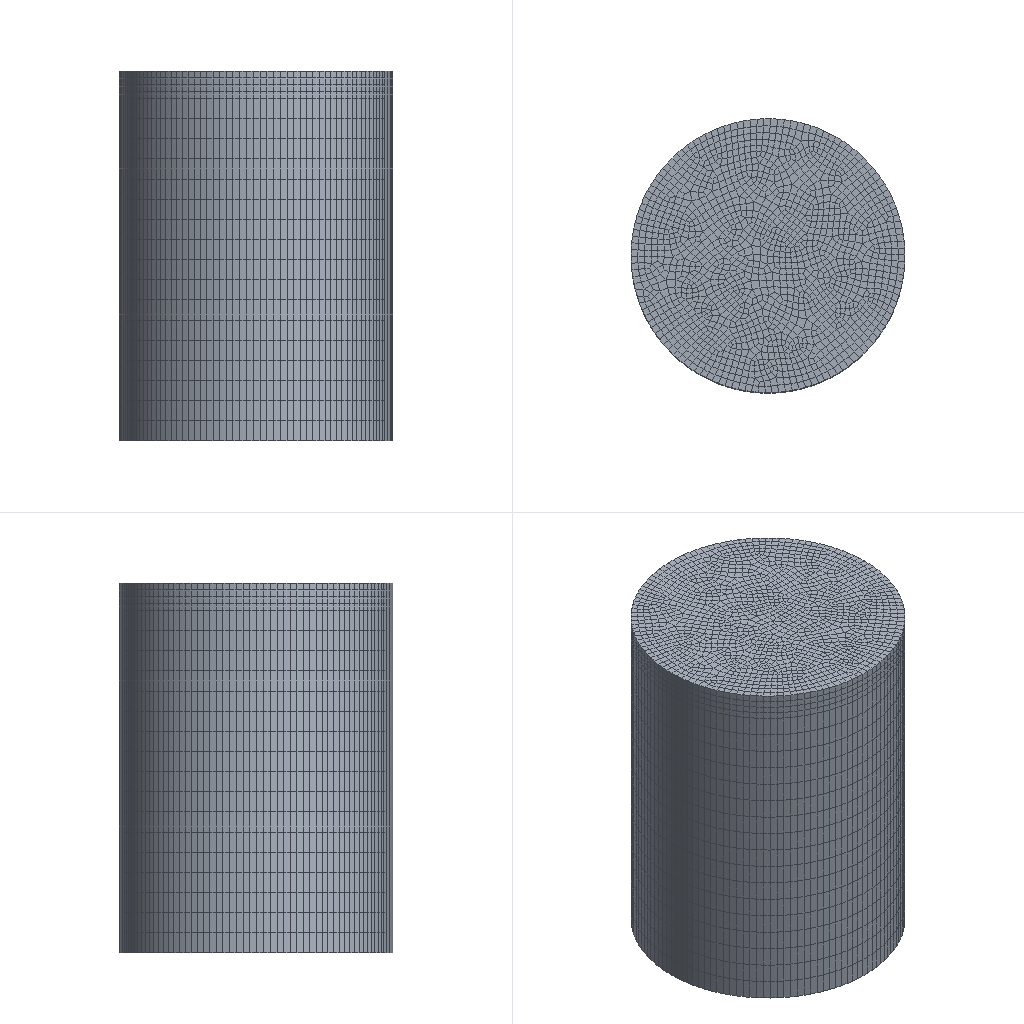Simulation study | abaqus
Set-up summary:
category,name,step,type,value,unit,region
solver,abaqus
solver,version,,,Abaqus/Explicit 2020
units,not stated in the deck,,not stated
analysis,deck,,transient,transient
load_step,Step-1,Step-1,transient
load_step,requested,,,1
mesh,nodes,,,37413
mesh,elements,,,34494
element_type,R3D3,,rigid,192
element_type,R3D4,,rigid,618
element_type,C3D8R,,solid,33684
load,load commands in deck,,count,2
bc,support commands in deck,,count,7
material,AL,,in results
material,CFRP-COPY,,in results
check,setup vs results,,match,"per instance, exact: element labels, types and connectivity; labels of the nodes the elements use; coordinates not compared"
Abaqus input file, long lists of numbers shortened:
*Heading
** Job name: Job-2 Model name: Model-1-Copy
** Generated by: Abaqus/CAE 2020
*Preprint, echo=NO, model=NO, history=NO, contact=NO
**
** PARTS
**
*Part, name=work
*Node
      1,   1.6,  -1.2,   5.2
      2,   1.6,  -1.2,    5.1
** (36694 more lines like these left out)
*Element, type=C3D8R
   1, 1117, 1163, 1135, 1050, 2659, 2705, 2677, 2592
   2,   81, 1117, 1050,   80,  206, 2659, 2592,  205
** (33682 more lines like these left out)
*Nset, nset=Set-18
     3,     4,   257,   258,   259,   260,   261,   262,   263,   264,   265,   266,   267,   268,   269,   270
   271,   272,   273,   274,   275,   276,   277,   278,   279,   280,   281,   282,   283,   284,   285,   286
** (1875 more lines like these left out)
*Elset, elset=Set-18, generate
  3209,  30476,      1
*Nset, nset=Set-17
     1,     2,     5,     6,     7,     8,     9,    10,    11,    12,    13,    14,    15,    16,    17,    18
    19,    20,    21,    22,    23,    24,    25,    26,    27,    28,    29,    30,    31,    32,    33,    34
** (415 more lines like these left out)
*Elset, elset=Set-17
     1,     2,     3,     4,     5,     6,     7,     8,     9,    10,    11,    12,    13,    14,    15,    16
    17,    18,    19,    20,    21,    22,    23,    24,    25,    26,    27,    28,    29,    30,    31,    32
** (299 more lines like these left out)
*Nset, nset=Set-19
     1,     2,     3,     5,     6,     7,     8,     9,    10,    11,    12,    13,    14,    15,    16,    17
    18,    19,    20,    21,    22,    23,    24,    25,    26,    27,    28,    29,    30,    31,    32,    33
** (520 more lines like these left out)
*Elset, elset=Set-19
     1,     2,     3,     4,     5,     6,     7,     8,     9,    10,    11,    12,    13,    14,    15,    16
    17,    18,    19,    20,    21,    22,    23,    24,    25,    26,    27,    28,    29,    30,    31,    32
** (399 more lines like these left out)
** Section: Section-2
*Solid Section, elset=Set-19, material=cfrp-Copy
,
** Section: al
*Solid Section, elset=Set-18, material=al
,
*End Part
**
*Part, name=zuantou_tool
*Node
      1,   0.8975, -0.3369,  0.4764
      2,  0.9447, -0.3279,  0.4373
** (714 more lines like these left out)
*Element, type=R3D4
 1,  1,  2, 34, 73
 2, 73, 34, 35, 72
** (616 more lines like these left out)
*Element, type=R3D3
371,  15,   4, 522
372, 537, 524, 527
** (190 more lines like these left out)
*Node
    717, -1.66533454e-16, -5.55111512e-17,   10.601
*Nset, nset=zuantou_tool-RefPt_, internal
717,
*Elset, elset=zuantou_tool, generate
   1,  810,    1
*End Part
**
**
** ASSEMBLY
**
*Assembly, name=Assembly
**
*Instance, name=work-1, part=work
*End Instance
**
*Instance, name=zuantou_tool-1, part=zuantou_tool
          0.,           0.,          5.4
*End Instance
**
*Node
      1,           0., 1.22464685e-16,           0.
*Nset, nset=Set-2, instance=zuantou_tool-1
 717,
*Nset, nset=Set-3, instance=zuantou_tool-1
 717,
*Nset, nset=Set-5, instance=zuantou_tool-1
 717,
*Nset, nset=Set-6, instance=work-1
    4,  382,  383,  384,  385,  386,  387,  388,  389,  390,  391,  392,  393,  394,  395,  396
  397,  398,  399,  400,  401,  402,  403,  404,  405,  406,  407,  408,  409,  410,  411,  412
** (103 more lines like these left out)
*Elset, elset=Set-6, instance=work-1, generate
 28873,  30476,      1
*Nset, nset=Set-7, instance=zuantou_tool-1
 717,
*Nset, nset=Set-11, instance=work-1
    4,  382,  383,  384,  385,  386,  387,  388,  389,  390,  391,  392,  393,  394,  395,  396
  397,  398,  399,  400,  401,  402,  403,  404,  405,  406,  407,  408,  409,  410,  411,  412
** (103 more lines like these left out)
*Elset, elset=Set-11, instance=work-1, generate
 28873,  30476,      1
*Nset, nset=m_Set-9
 1,
*Nset, nset=rp-fix
 1,
*Nset, nset=s_Set-4, instance=work-1
   4,   6, 382, 383, 384, 385, 386, 387, 388, 389, 390, 391, 392, 393, 394, 395
 396, 397, 398, 399, 400, 401, 402, 403, 404, 405, 406, 407, 408, 409, 410, 411
** (6 more lines like these left out)
*Elset, elset=s_Set-4, instance=work-1
 28874, 28885, 28888, 28900, 28901, 28912, 28913, 28922, 28923, 28926, 28927, 28928, 28934, 28947, 28950, 28951
 28952, 28954, 28966, 28981, 28988, 28989, 29014, 29015, 29031, 29032, 29039, 29042, 29045, 29048, 29050, 29051
** (6 more lines like these left out)
*Nset, nset=s_Set-8, instance=work-1, generate
     1,  36696,      1
*Elset, elset=s_Set-8, instance=work-1, generate
     1,  33684,      1
*Elset, elset=_m_Surf-1_SPOS, internal, instance=zuantou_tool-1, generate
   1,  810,    1
*Surface, type=ELEMENT, name=m_Surf-1
_m_Surf-1_SPOS, SPOS
*Elset, elset=_s_Surf-2_S2, internal, instance=work-1, generate
 28873,  30476,      1
*Surface, type=ELEMENT, name=s_Surf-2
_s_Surf-2_S2, S2
*Surface, type=NODE, name=s_Set-8_CNS_, internal
s_Set-8, 1.
*Rigid Body, ref node=zuantou_tool-1.zuantou_tool-RefPt_, elset=zuantou_tool-1.zuantou_tool
** Constraint: Constraint-1
*Coupling, constraint name=Constraint-1, ref node=m_Set-9, surface=s_Surf-2
*Kinematic
*End Assembly
*Amplitude, name=Amp-1, definition=PERIODIC
1,         251200.,              0.,            -10.
         3265.6,              0.
**
** MATERIALS
**
*Material, name=al
*Conductivity
188.,
*Damage Initiation, criterion=JOHNSON COOK
 -0.77,  1.45, -0.47,    0.,   1.6,  790.,  293.,    1.
*Damage Evolution, type=DISPLACEMENT
 0.001,
*Density
 2.7e-09,
*Elastic
70000., 0.33
*Plastic, hardening=JOHNSON COOK
324., 114., 0.42, 1.34, 790., 293.
*Rate Dependent, type=JOHNSON COOK
 0.002,1.
*Specific Heat
 8.9e+08,
*Material, name=cfrp-Copy
*Damage Initiation, criterion=SHEAR
 0.01, 0.8, 0.2
*Damage Evolution, type=DISPLACEMENT
 0.001,
*Density
 1.6e-09,
*Elastic
153000., 0.2
*Plastic
100.,0.
**
** INTERACTION PROPERTIES
**
*Surface Interaction, name=IntProp-1
*Friction
 0.3,
*Surface Behavior, pressure-overclosure=HARD
**
** BOUNDARY CONDITIONS
**
** Name: BC-1 Type: 对称/反对称/完全固定
*Boundary
Set-11, ENCASTRE
** ----------------------------------------------------------------
**
** STEP: Step-1
**
*Step, name=Step-1, nlgeom=YES
*Dynamic, Explicit
, 0.5
*Bulk Viscosity
0.06, 1.2
** Mass Scaling: Semi-Automatic
**               Whole Model
*Fixed Mass Scaling, factor=5000.
**
** BOUNDARY CONDITIONS
**
** Name: BC-3 Type: 速度/角速度
*Boundary, type=VELOCITY
Set-7, 1, 1
Set-7, 2, 2
Set-7, 4, 4
Set-7, 5, 5
Set-7, 6, 6, -314.
** Name: [REDACTED] : Velocity/Angular velocity
*Boundary, amplitude=Amp-1, type=VELOCITY
Set-2, 3, 3, 1.
**
** INTERACTIONS
**
** Interaction: Int-1
*Contact Pair, interaction=IntProp-1, mechanical constraint=KINEMATIC, cpset=Int-1
m_Surf-1, s_Set-8_CNS_
** Interaction: Int-2
*Contact, op=NEW
*Contact Inclusions, ALL EXTERIOR
*Contact Property Assignment
 ,  , IntProp-1
**
** OUTPUT REQUESTS
**
*Restart, write, number interval=1, time marks=NO
**
** FIELD OUTPUT: F-Output-1
**
*Output, field, number interval=150
*Node Output
A, RF, U, V
*Element Output, directions=YES
DAMAGEC, DAMAGEFC, DAMAGEFT, DAMAGEMC, DAMAGEMT, DAMAGET, DMICRT, E, LE, MISES, PE, PEEQ, PEEQVAVG, PEVAVG, S, SDEG
STATUS, SVAVG
*Contact Output
CSTRESS,
**
** HISTORY OUTPUT: H-Output-3
**
*Output, history, time interval=0.0005
*Contact Output, cpset=Int-1
CFN1, CFN2, CFN3, CFNM, CFS1, CFS2, CFS3, CFSM, CFT1, CFT2, CFT3, CFTM, CMN1, CMN2, CMN3, CMNM
CMS1, CMS2, CMS3, CMSM, CMT1, CMT2, CMT3, CMTM
**
** HISTORY OUTPUT: H-Output-1
**
*Node Output, nset=Set-2
RF1, RF2, RF3, RM1, RM2, RM3
**
** HISTORY OUTPUT: H-Output-2
**
*Contact Output, surface=m_Surf-1
CFN1, CFN2, CFN3, CFNM, CFS1, CFS2, CFS3, CFSM, CFT1, CFT2, CFT3, CFTM, CMN1, CMN2, CMN3, CMNM
CMS1, CMS2, CMS3, CMSM, CMT1, CMT2, CMT3, CMTM
**
** HISTORY OUTPUT: H-Output-5
**
*Output, history, time interval=0.00025
*Node Output, nset=Set-11
CF1, CF2, CF3, CM1, CM2, CM3, RF1, RF2
RF3, RM1, RM2, RM3
*Element Output, elset=Set-11
SF1, SF2, SF3, SM1, SM2, SM3
**
** HISTORY OUTPUT: H-Output-4
**
*Node Output, nset=rp-fix
CF1, CF2, CF3, CM1, CM2, CM3, RF1, RF2
RF3, RM1, RM2, RM3
*End Step
Results summary:
result,step,Step-1,partial,increments=787408 time=0.2925/0.5
result,analysis,,,transient
result,last_loadstep,,,1
result,primary field,,,U
result,reaction total,,FX,30.604,model units
result,reaction total,,FY,-5.107,model units
result,reaction total,,FZ,62.971,model units